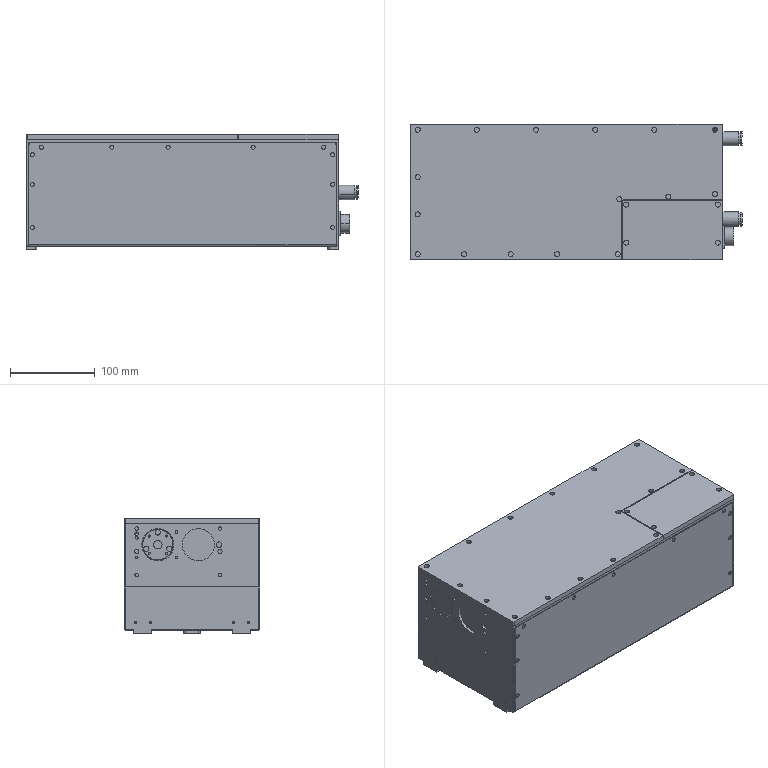Part | STEP file | 族光1号紫外激光器三维模型图202110 | 2 solids | 1075 faces | box 392.5 x 160 x 136 mm | volume 7837982 mm3 | spline 1071 | cylinder 2 | plane 2 | commonest cylinder face diameters 36 x2